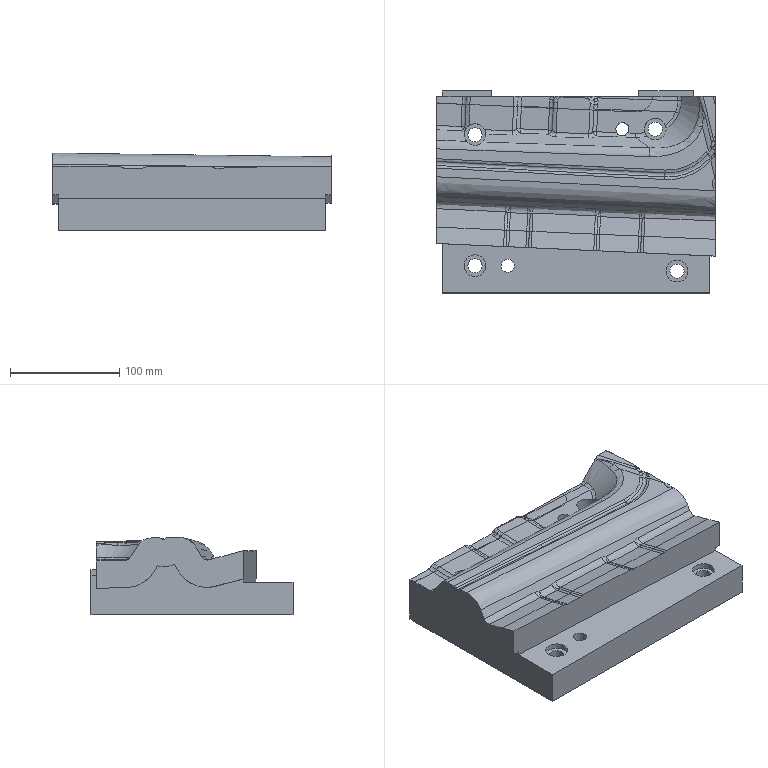Part | NX | features solid 2 | 1 solid | 190 faces | box 255.001 x 185 x 71.276 mm | volume 2331595 mm3 | spline 159 | plane 21 | cylinder 10 | commonest cylinder face diameters 13 x4 20 x4 12 x2